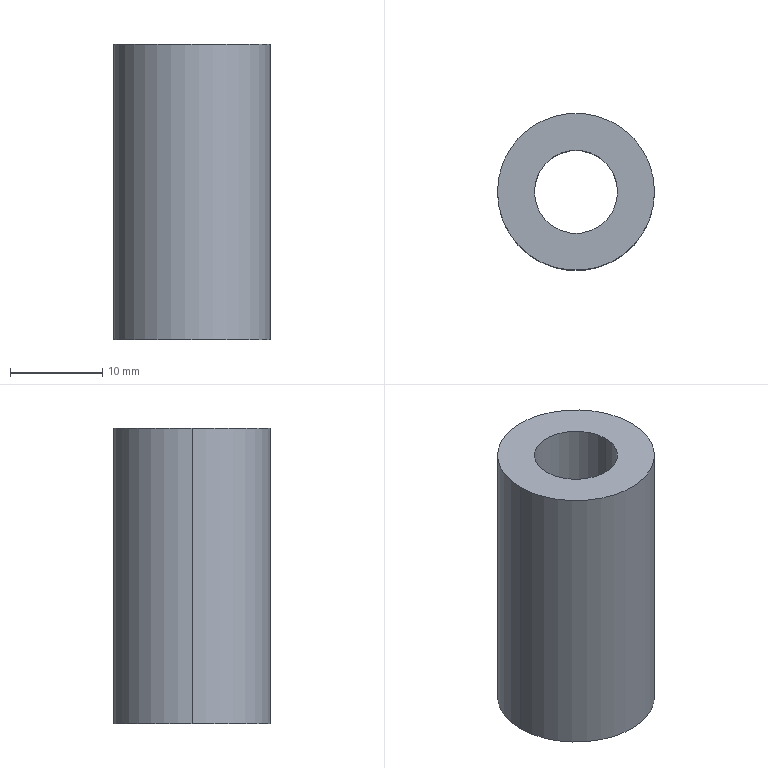Part | SolidWorks | features Extrusion 1 | 1 solid | 6 faces | box 17 x 17 x 32 mm | volume 5228 mm3 | cylinder 4 | plane 2 | commonest cylinder face diameters 9 x2 17 x2
STEP:
#1=CARTESIAN_POINT('',(-4.5,0.,32.));
#2=VERTEX_POINT('',#1);
#3=CARTESIAN_POINT('',(4.5,0.,32.));
#4=VERTEX_POINT('',#3);
#5=CARTESIAN_POINT('',(0.,0.,32.));
#6=DIRECTION('',(0.,0.,1.));
#7=DIRECTION('',(1.,0.,0.));
#8=AXIS2_PLACEMENT_3D('',#5,#6,#7);
#9=CIRCLE('',#8,4.5);
#10=EDGE_CURVE('',#2,#4,#9,.T.);
#11=ORIENTED_EDGE('',*,*,#10,.T.);
#12=CARTESIAN_POINT('',(4.5,0.,0.));
#13=VERTEX_POINT('',#12);
#14=CARTESIAN_POINT('',(4.5,0.,32.));
#15=DIRECTION('',(0.,0.,-1.));
#16=VECTOR('',#15,1000.);
#17=LINE('',#14,#16);
#18=EDGE_CURVE('',#4,#13,#17,.T.);
#19=ORIENTED_EDGE('',*,*,#18,.T.);
#20=CARTESIAN_POINT('',(-4.5,0.,0.));
#21=VERTEX_POINT('',#20);
#22=CARTESIAN_POINT('',(0.,0.,0.));
#23=DIRECTION('',(0.,0.,1.));
#24=DIRECTION('',(1.,0.,0.));
#25=AXIS2_PLACEMENT_3D('',#22,#23,#24);
#26=CIRCLE('',#25,4.5);
#27=EDGE_CURVE('',#21,#13,#26,.T.);
#28=ORIENTED_EDGE('',*,*,#27,.F.);
#29=CARTESIAN_POINT('',(-4.5,0.,32.));
#30=DIRECTION('',(0.,0.,-1.));
#31=VECTOR('',#30,1000.);
#32=LINE('',#29,#31);
#33=EDGE_CURVE('',#2,#21,#32,.T.);
#34=ORIENTED_EDGE('',*,*,#33,.F.);
#35=EDGE_LOOP('',(#11,#19,#28,#34));
#36=FACE_OUTER_BOUND('',#35,.T.);
#37=CARTESIAN_POINT('',(0.,0.,32.));
#38=DIRECTION('',(0.,0.,-1.));
#39=DIRECTION('',(-1.,0.,0.));
#40=AXIS2_PLACEMENT_3D('',#37,#38,#39);
#41=CYLINDRICAL_SURFACE('',#40,4.5);
#42=ADVANCED_FACE('',(#36),#41,.F.);
#43=CARTESIAN_POINT('',(8.5,0.,32.));
#44=VERTEX_POINT('',#43);
#45=CARTESIAN_POINT('',(-8.5,0.,32.));
#46=VERTEX_POINT('',#45);
#47=CARTESIAN_POINT('',(0.,0.,32.));
#48=DIRECTION('',(0.,0.,1.));
#49=DIRECTION('',(1.,0.,0.));
#50=AXIS2_PLACEMENT_3D('',#47,#48,#49);
#51=CIRCLE('',#50,8.5);
#52=EDGE_CURVE('',#44,#46,#51,.T.);
#53=ORIENTED_EDGE('',*,*,#52,.F.);
#54=CARTESIAN_POINT('',(8.5,0.,0.));
#55=VERTEX_POINT('',#54);
#56=CARTESIAN_POINT('',(8.5,0.,32.));
#57=DIRECTION('',(0.,0.,-1.));
#58=VECTOR('',#57,1000.);
#59=LINE('',#56,#58);
#60=EDGE_CURVE('',#44,#55,#59,.T.);
#61=ORIENTED_EDGE('',*,*,#60,.T.);
#62=CARTESIAN_POINT('',(-8.5,0.,0.));
#63=VERTEX_POINT('',#62);
#64=CARTESIAN_POINT('',(0.,0.,0.));
#65=DIRECTION('',(0.,0.,1.));
#66=DIRECTION('',(1.,0.,0.));
#67=AXIS2_PLACEMENT_3D('',#64,#65,#66);
#68=CIRCLE('',#67,8.5);
#69=EDGE_CURVE('',#55,#63,#68,.T.);
#70=ORIENTED_EDGE('',*,*,#69,.T.);
#71=CARTESIAN_POINT('',(-8.5,0.,32.));
#72=DIRECTION('',(0.,0.,-1.));
#73=VECTOR('',#72,1000.);
#74=LINE('',#71,#73);
#75=EDGE_CURVE('',#46,#63,#74,.T.);
#76=ORIENTED_EDGE('',*,*,#75,.F.);
#77=EDGE_LOOP('',(#53,#61,#70,#76));
#78=FACE_OUTER_BOUND('',#77,.T.);
#79=CARTESIAN_POINT('',(0.,0.,32.));
#80=DIRECTION('',(0.,0.,-1.));
#81=DIRECTION('',(-1.,0.,0.));
#82=AXIS2_PLACEMENT_3D('',#79,#80,#81);
#83=CYLINDRICAL_SURFACE('',#82,8.5);
#84=ADVANCED_FACE('',(#78),#83,.T.);
#85=CARTESIAN_POINT('',(0.,0.,32.));
#86=DIRECTION('',(0.,0.,1.));
#87=DIRECTION('',(1.,0.,0.));
#88=AXIS2_PLACEMENT_3D('',#85,#86,#87);
#89=CIRCLE('',#88,8.5);
#90=EDGE_CURVE('',#46,#44,#89,.T.);
#91=ORIENTED_EDGE('',*,*,#90,.T.);
#92=ORIENTED_EDGE('',*,*,#52,.T.);
#93=EDGE_LOOP('',(#91,#92));
#94=FACE_OUTER_BOUND('',#93,.T.);
#95=ORIENTED_EDGE('',*,*,#10,.F.);
#96=CARTESIAN_POINT('',(0.,0.,32.));
#97=DIRECTION('',(0.,0.,1.));
#98=DIRECTION('',(1.,0.,0.));
#99=AXIS2_PLACEMENT_3D('',#96,#97,#98);
#100=CIRCLE('',#99,4.5);
#101=EDGE_CURVE('',#4,#2,#100,.T.);
#102=ORIENTED_EDGE('',*,*,#101,.F.);
#103=EDGE_LOOP('',(#95,#102));
#104=FACE_BOUND('',#103,.T.);
#105=CARTESIAN_POINT('',(0.,0.,32.));
#106=DIRECTION('',(0.,0.,1.));
#107=DIRECTION('',(1.,0.,0.));
#108=AXIS2_PLACEMENT_3D('',#105,#106,#107);
#109=PLANE('',#108);
#110=ADVANCED_FACE('',(#94,#104),#109,.T.);
#111=CARTESIAN_POINT('',(0.,0.,0.));
#112=DIRECTION('',(0.,0.,1.));
#113=DIRECTION('',(1.,0.,0.));
#114=AXIS2_PLACEMENT_3D('',#111,#112,#113);
#115=CIRCLE('',#114,8.5);
#116=EDGE_CURVE('',#63,#55,#115,.T.);
#117=ORIENTED_EDGE('',*,*,#116,.F.);
#118=ORIENTED_EDGE('',*,*,#69,.F.);
#119=EDGE_LOOP('',(#117,#118));
#120=FACE_OUTER_BOUND('',#119,.T.);
#121=ORIENTED_EDGE('',*,*,#27,.T.);
#122=CARTESIAN_POINT('',(0.,0.,0.));
#123=DIRECTION('',(0.,0.,1.));
#124=DIRECTION('',(1.,0.,0.));
#125=AXIS2_PLACEMENT_3D('',#122,#123,#124);
#126=CIRCLE('',#125,4.5);
#127=EDGE_CURVE('',#13,#21,#126,.T.);
#128=ORIENTED_EDGE('',*,*,#127,.T.);
#129=EDGE_LOOP('',(#121,#128));
#130=FACE_BOUND('',#129,.T.);
#131=CARTESIAN_POINT('',(0.,0.,0.));
#132=DIRECTION('',(0.,0.,1.));
#133=DIRECTION('',(1.,0.,0.));
#134=AXIS2_PLACEMENT_3D('',#131,#132,#133);
#135=PLANE('',#134);
#136=ADVANCED_FACE('',(#120,#130),#135,.F.);
#137=ORIENTED_EDGE('',*,*,#60,.F.);
#138=ORIENTED_EDGE('',*,*,#90,.F.);
#139=ORIENTED_EDGE('',*,*,#75,.T.);
#140=ORIENTED_EDGE('',*,*,#116,.T.);
#141=EDGE_LOOP('',(#137,#138,#139,#140));
#142=FACE_OUTER_BOUND('',#141,.T.);
#143=CARTESIAN_POINT('',(0.,0.,32.));
#144=DIRECTION('',(0.,0.,-1.));
#145=DIRECTION('',(-1.,0.,0.));
#146=AXIS2_PLACEMENT_3D('',#143,#144,#145);
#147=CYLINDRICAL_SURFACE('',#146,8.5);
#148=ADVANCED_FACE('',(#142),#147,.T.);
#149=ORIENTED_EDGE('',*,*,#18,.F.);
#150=ORIENTED_EDGE('',*,*,#101,.T.);
#151=ORIENTED_EDGE('',*,*,#33,.T.);
#152=ORIENTED_EDGE('',*,*,#127,.F.);
#153=EDGE_LOOP('',(#149,#150,#151,#152));
#154=FACE_OUTER_BOUND('',#153,.T.);
#155=CARTESIAN_POINT('',(0.,0.,32.));
#156=DIRECTION('',(0.,0.,-1.));
#157=DIRECTION('',(-1.,0.,0.));
#158=AXIS2_PLACEMENT_3D('',#155,#156,#157);
#159=CYLINDRICAL_SURFACE('',#158,4.5);
#160=ADVANCED_FACE('',(#154),#159,.F.);
#161=CLOSED_SHELL('',(#42,#84,#110,#136,#148,#160));
#162=MANIFOLD_SOLID_BREP('',#161);
#163=CARTESIAN_POINT('',(0.,0.,0.));
#164=DIRECTION('',(0.,0.,1.));
#165=DIRECTION('',(1.,0.,0.));
#166=AXIS2_PLACEMENT_3D('',#163,#164,#165);
#167=(LENGTH_UNIT()NAMED_UNIT(*)SI_UNIT(.MILLI.,.METRE.));
#168=UNCERTAINTY_MEASURE_WITH_UNIT(LENGTH_MEASURE(0.00001),#167,'','');
#169=(NAMED_UNIT(*)PLANE_ANGLE_UNIT()SI_UNIT($,.RADIAN.));
#170=(NAMED_UNIT(*)SI_UNIT($,.STERADIAN.)SOLID_ANGLE_UNIT());
#171=(GEOMETRIC_REPRESENTATION_CONTEXT(3)GLOBAL_UNCERTAINTY_ASSIGNED_CONTEXT((#168))GLOBAL_UNIT_ASSIGNED_CONTEXT((#167,#169,#170))REPRESENTATION_CONTEXT('',''));
#172=ADVANCED_BREP_SHAPE_REPRESENTATION('',(#162,#166),#171);